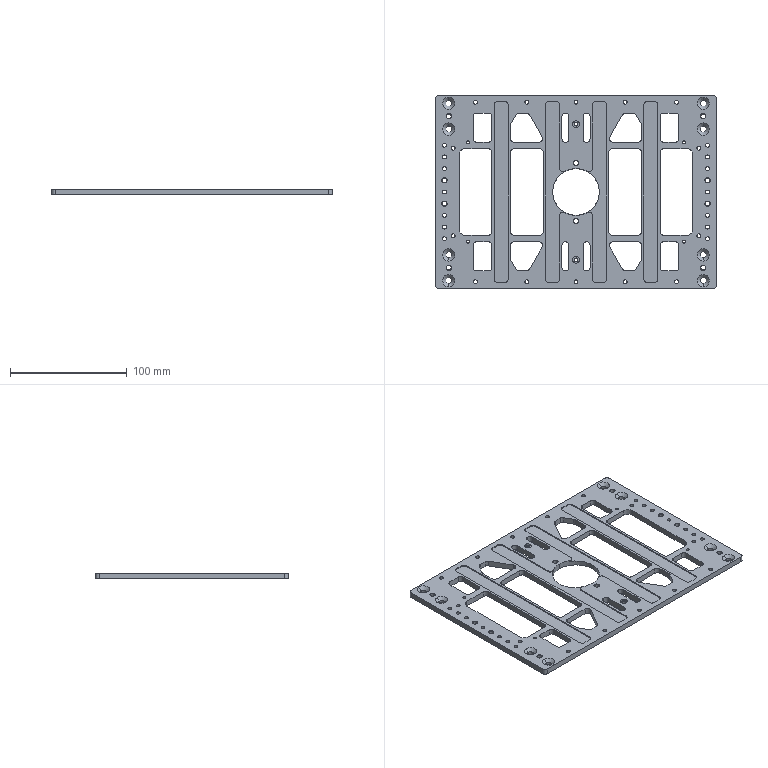Part | 1 solid | 346 faces | box 240 x 165 x 5 mm | volume 119272 mm3 | cylinder 200 | plane 90 | cone 56 | commonest cylinder face diameters 6 x90 3.3 x56 4 x20 5.3 x16 2.5 x8 3.2 x4